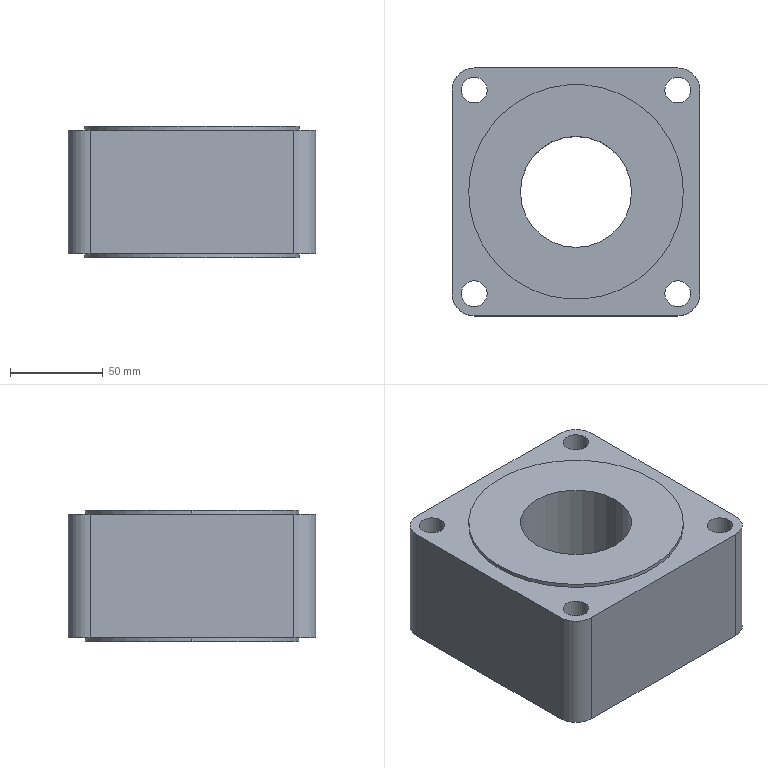Part | SolidWorks | features ICE 5, HoleWzd 3, Extrusion 1, Fillet 1 | 1 solid | 78 faces | box 134 x 134 x 71 mm | volume 961535 mm3 | cylinder 46 | cone 20 | plane 12 | commonest cylinder face diameters 8.5 x16 14 x8 19 x8 8.6 x4 24 x4 116 x4